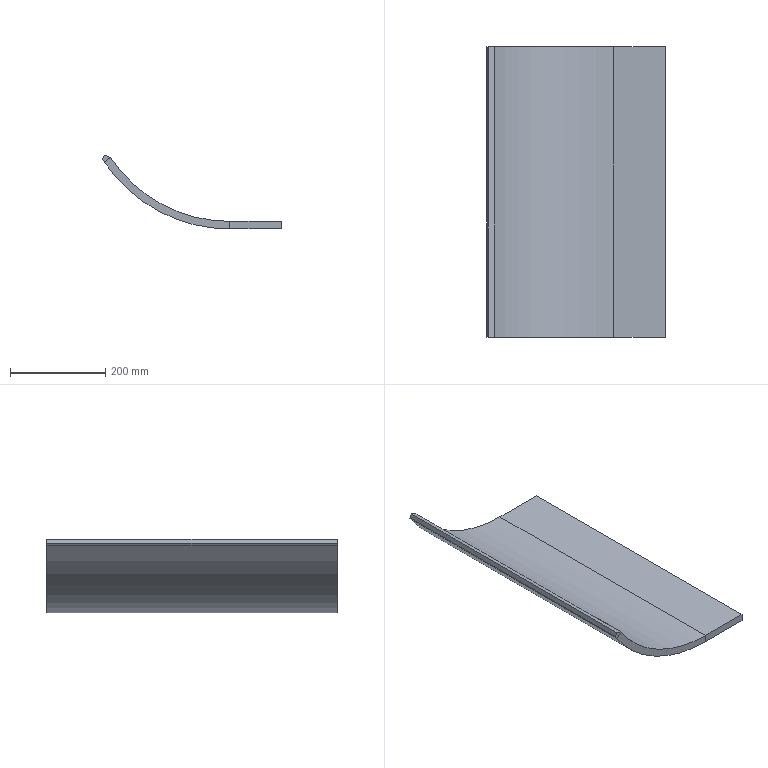Part | SolidWorks | features Chamfer 2, FlatPattern 1, SM3dBend 1, SMBaseFlange 1, SheetMetal 1 | 1 solid | 15 faces | box 375.791 x 610 x 155.275 mm | volume 4096516 mm3 | plane 13 | cylinder 2 | commonest cylinder face diameters 602 x1 634 x1
STEP:
#1=CARTESIAN_POINT('',(64.897,610.,133.992));
#2=VERTEX_POINT('',#1);
#3=CARTESIAN_POINT('',(64.794,610.,134.146));
#4=VERTEX_POINT('',#3);
#5=CARTESIAN_POINT('',(58.413,610.,143.713));
#6=DIRECTION('',(-0.5548,0.,0.832));
#7=VECTOR('',#6,1000.);
#8=LINE('',#5,#7);
#9=EDGE_CURVE('',#2,#4,#8,.T.);
#10=ORIENTED_EDGE('',*,*,#9,.F.);
#11=CARTESIAN_POINT('',(51.585,610.,125.114));
#12=VERTEX_POINT('',#11);
#13=CARTESIAN_POINT('',(51.585,610.,125.114));
#14=DIRECTION('',(-0.832,0.,-0.5548));
#15=VECTOR('',#14,1000.);
#16=LINE('',#13,#15);
#17=EDGE_CURVE('',#2,#12,#16,.T.);
#18=ORIENTED_EDGE('',*,*,#17,.T.);
#19=CARTESIAN_POINT('',(48.209,610.,130.177));
#20=VERTEX_POINT('',#19);
#21=CARTESIAN_POINT('',(45.102,610.,134.836));
#22=DIRECTION('',(-0.5548,0.,0.832));
#23=VECTOR('',#22,1000.);
#24=LINE('',#21,#23);
#25=EDGE_CURVE('',#12,#20,#24,.T.);
#26=ORIENTED_EDGE('',*,*,#25,.T.);
#27=CARTESIAN_POINT('',(51.758,610.,139.275));
#28=VERTEX_POINT('',#27);
#29=CARTESIAN_POINT('',(49.376,610.,133.169));
#30=DIRECTION('',(0.3634,0.,0.9316));
#31=VECTOR('',#30,1000.);
#32=LINE('',#29,#31);
#33=EDGE_CURVE('',#20,#28,#32,.T.);
#34=ORIENTED_EDGE('',*,*,#33,.T.);
#35=CARTESIAN_POINT('',(47.506,610.,140.947));
#36=DIRECTION('',(0.9306,0.,-0.3661));
#37=VECTOR('',#36,1000.);
#38=LINE('',#35,#37);
#39=EDGE_CURVE('',#28,#4,#38,.T.);
#40=ORIENTED_EDGE('',*,*,#39,.T.);
#41=EDGE_LOOP('',(#10,#18,#26,#34,#40));
#42=FACE_OUTER_BOUND('',#41,.T.);
#43=CARTESIAN_POINT('',(45.102,610.,134.836));
#44=DIRECTION('',(0.,1.,0.));
#45=DIRECTION('',(0.832,0.,0.5548));
#46=AXIS2_PLACEMENT_3D('',#43,#44,#45);
#47=PLANE('',#46);
#48=ADVANCED_FACE('',(#42),#47,.T.);
#49=CARTESIAN_POINT('',(48.209,0.,130.177));
#50=VERTEX_POINT('',#49);
#51=CARTESIAN_POINT('',(51.585,0.,125.114));
#52=VERTEX_POINT('',#51);
#53=CARTESIAN_POINT('',(45.102,0.,134.836));
#54=DIRECTION('',(0.5548,0.,-0.832));
#55=VECTOR('',#54,1000.);
#56=LINE('',#53,#55);
#57=EDGE_CURVE('',#50,#52,#56,.T.);
#58=ORIENTED_EDGE('',*,*,#57,.T.);
#59=CARTESIAN_POINT('',(64.897,0.,133.992));
#60=VERTEX_POINT('',#59);
#61=CARTESIAN_POINT('',(51.585,0.,125.114));
#62=DIRECTION('',(0.832,0.,0.5548));
#63=VECTOR('',#62,1000.);
#64=LINE('',#61,#63);
#65=EDGE_CURVE('',#52,#60,#64,.T.);
#66=ORIENTED_EDGE('',*,*,#65,.T.);
#67=CARTESIAN_POINT('',(64.794,0.,134.146));
#68=VERTEX_POINT('',#67);
#69=CARTESIAN_POINT('',(58.413,0.,143.713));
#70=DIRECTION('',(0.5548,0.,-0.832));
#71=VECTOR('',#70,1000.);
#72=LINE('',#69,#71);
#73=EDGE_CURVE('',#68,#60,#72,.T.);
#74=ORIENTED_EDGE('',*,*,#73,.F.);
#75=CARTESIAN_POINT('',(51.758,0.,139.275));
#76=VERTEX_POINT('',#75);
#77=CARTESIAN_POINT('',(47.506,0.,140.947));
#78=DIRECTION('',(-0.9306,0.,0.3661));
#79=VECTOR('',#78,1000.);
#80=LINE('',#77,#79);
#81=EDGE_CURVE('',#68,#76,#80,.T.);
#82=ORIENTED_EDGE('',*,*,#81,.T.);
#83=CARTESIAN_POINT('',(49.376,0.,133.169));
#84=DIRECTION('',(-0.3634,0.,-0.9316));
#85=VECTOR('',#84,1000.);
#86=LINE('',#83,#85);
#87=EDGE_CURVE('',#76,#50,#86,.T.);
#88=ORIENTED_EDGE('',*,*,#87,.T.);
#89=EDGE_LOOP('',(#58,#66,#74,#82,#88));
#90=FACE_OUTER_BOUND('',#89,.T.);
#91=CARTESIAN_POINT('',(45.102,0.,134.836));
#92=DIRECTION('',(0.,-1.,0.));
#93=DIRECTION('',(-0.832,0.,-0.5548));
#94=AXIS2_PLACEMENT_3D('',#91,#92,#93);
#95=PLANE('',#94);
#96=ADVANCED_FACE('',(#90),#95,.T.);
#97=ORIENTED_EDGE('',*,*,#25,.F.);
#98=CARTESIAN_POINT('',(51.585,610.,125.114));
#99=DIRECTION('',(0.,-1.,0.));
#100=VECTOR('',#99,1000.);
#101=LINE('',#98,#100);
#102=EDGE_CURVE('',#12,#52,#101,.T.);
#103=ORIENTED_EDGE('',*,*,#102,.T.);
#104=ORIENTED_EDGE('',*,*,#57,.F.);
#105=CARTESIAN_POINT('',(48.209,610.,130.177));
#106=DIRECTION('',(0.,1.,0.));
#107=VECTOR('',#106,1000.);
#108=LINE('',#105,#107);
#109=EDGE_CURVE('',#50,#20,#108,.T.);
#110=ORIENTED_EDGE('',*,*,#109,.T.);
#111=EDGE_LOOP('',(#97,#103,#104,#110));
#112=FACE_OUTER_BOUND('',#111,.T.);
#113=CARTESIAN_POINT('',(45.102,610.,134.836));
#114=DIRECTION('',(-0.832,0.,-0.5548));
#115=DIRECTION('',(-0.5548,0.,0.832));
#116=AXIS2_PLACEMENT_3D('',#113,#114,#115);
#117=PLANE('',#116);
#118=ADVANCED_FACE('',(#112),#117,.T.);
#119=CARTESIAN_POINT('',(64.897,610.,133.992));
#120=DIRECTION('',(0.,-1.,0.));
#121=VECTOR('',#120,1000.);
#122=LINE('',#119,#121);
#123=EDGE_CURVE('',#2,#60,#122,.T.);
#124=ORIENTED_EDGE('',*,*,#123,.F.);
#125=ORIENTED_EDGE('',*,*,#9,.T.);
#126=CARTESIAN_POINT('',(64.794,0.,134.146));
#127=DIRECTION('',(0.,-1.,0.));
#128=VECTOR('',#127,1000.);
#129=LINE('',#126,#128);
#130=EDGE_CURVE('',#4,#68,#129,.T.);
#131=ORIENTED_EDGE('',*,*,#130,.T.);
#132=ORIENTED_EDGE('',*,*,#73,.T.);
#133=EDGE_LOOP('',(#124,#125,#131,#132));
#134=FACE_OUTER_BOUND('',#133,.T.);
#135=CARTESIAN_POINT('',(58.413,610.,143.713));
#136=DIRECTION('',(-0.832,0.,-0.5548));
#137=DIRECTION('',(-0.5548,0.,0.832));
#138=AXIS2_PLACEMENT_3D('',#135,#136,#137);
#139=PLANE('',#138);
#140=ADVANCED_FACE('',(#134),#139,.F.);
#141=ORIENTED_EDGE('',*,*,#39,.F.);
#142=CARTESIAN_POINT('',(51.758,610.,139.275));
#143=DIRECTION('',(0.,1.,0.));
#144=VECTOR('',#143,1000.);
#145=LINE('',#142,#144);
#146=EDGE_CURVE('',#76,#28,#145,.T.);
#147=ORIENTED_EDGE('',*,*,#146,.F.);
#148=ORIENTED_EDGE('',*,*,#81,.F.);
#149=ORIENTED_EDGE('',*,*,#130,.F.);
#150=EDGE_LOOP('',(#141,#147,#148,#149));
#151=FACE_OUTER_BOUND('',#150,.T.);
#152=CARTESIAN_POINT('',(64.794,610.,134.146));
#153=DIRECTION('',(0.3661,0.,0.9306));
#154=DIRECTION('',(0.9306,0.,-0.3661));
#155=AXIS2_PLACEMENT_3D('',#152,#153,#154);
#156=PLANE('',#155);
#157=ADVANCED_FACE('',(#151),#156,.T.);
#158=ORIENTED_EDGE('',*,*,#33,.F.);
#159=ORIENTED_EDGE('',*,*,#109,.F.);
#160=ORIENTED_EDGE('',*,*,#87,.F.);
#161=ORIENTED_EDGE('',*,*,#146,.T.);
#162=EDGE_LOOP('',(#158,#159,#160,#161));
#163=FACE_OUTER_BOUND('',#162,.T.);
#164=CARTESIAN_POINT('',(51.758,0.,139.275));
#165=DIRECTION('',(0.9316,0.,-0.3634));
#166=DIRECTION('',(-0.3634,0.,-0.9316));
#167=AXIS2_PLACEMENT_3D('',#164,#165,#166);
#168=PLANE('',#167);
#169=ADVANCED_FACE('',(#163),#168,.F.);
#170=CARTESIAN_POINT('',(424.,0.,0.));
#171=VERTEX_POINT('',#170);
#172=CARTESIAN_POINT('',(424.,610.,0.));
#173=VERTEX_POINT('',#172);
#174=CARTESIAN_POINT('',(424.,0.,0.));
#175=DIRECTION('',(0.,1.,0.));
#176=VECTOR('',#175,1000.);
#177=LINE('',#174,#176);
#178=EDGE_CURVE('',#171,#173,#177,.T.);
#179=ORIENTED_EDGE('',*,*,#178,.F.);
#180=CARTESIAN_POINT('',(424.,0.,-16.));
#181=VERTEX_POINT('',#180);
#182=CARTESIAN_POINT('',(424.,0.,-16.));
#183=DIRECTION('',(0.,0.,1.));
#184=VECTOR('',#183,1000.);
#185=LINE('',#182,#184);
#186=EDGE_CURVE('',#181,#171,#185,.T.);
#187=ORIENTED_EDGE('',*,*,#186,.F.);
#188=CARTESIAN_POINT('',(424.,610.,-16.));
#189=VERTEX_POINT('',#188);
#190=CARTESIAN_POINT('',(424.,0.,-16.));
#191=DIRECTION('',(0.,1.,0.));
#192=VECTOR('',#191,1000.);
#193=LINE('',#190,#192);
#194=EDGE_CURVE('',#181,#189,#193,.T.);
#195=ORIENTED_EDGE('',*,*,#194,.T.);
#196=CARTESIAN_POINT('',(424.,610.,-16.));
#197=DIRECTION('',(0.,0.,1.));
#198=VECTOR('',#197,1000.);
#199=LINE('',#196,#198);
#200=EDGE_CURVE('',#189,#173,#199,.T.);
#201=ORIENTED_EDGE('',*,*,#200,.T.);
#202=EDGE_LOOP('',(#179,#187,#195,#201));
#203=FACE_OUTER_BOUND('',#202,.T.);
#204=CARTESIAN_POINT('',(424.,0.,-16.));
#205=DIRECTION('',(1.,0.,0.));
#206=DIRECTION('',(0.,0.,-1.));
#207=AXIS2_PLACEMENT_3D('',#204,#205,#206);
#208=PLANE('',#207);
#209=ADVANCED_FACE('',(#203),#208,.T.);
#210=CARTESIAN_POINT('',(315.315,610.,-16.));
#211=VERTEX_POINT('',#210);
#212=CARTESIAN_POINT('',(315.315,0.,-16.));
#213=VERTEX_POINT('',#212);
#214=CARTESIAN_POINT('',(315.315,610.,-16.));
#215=DIRECTION('',(0.,-1.,0.));
#216=VECTOR('',#215,1000.);
#217=LINE('',#214,#216);
#218=EDGE_CURVE('',#211,#213,#217,.T.);
#219=ORIENTED_EDGE('',*,*,#218,.F.);
#220=CARTESIAN_POINT('',(0.,610.,-16.));
#221=DIRECTION('',(-1.,0.,0.));
#222=VECTOR('',#221,1000.);
#223=LINE('',#220,#222);
#224=EDGE_CURVE('',#189,#211,#223,.T.);
#225=ORIENTED_EDGE('',*,*,#224,.F.);
#226=ORIENTED_EDGE('',*,*,#194,.F.);
#227=CARTESIAN_POINT('',(0.,0.,-16.));
#228=DIRECTION('',(1.,0.,0.));
#229=VECTOR('',#228,1000.);
#230=LINE('',#227,#229);
#231=EDGE_CURVE('',#213,#181,#230,.T.);
#232=ORIENTED_EDGE('',*,*,#231,.F.);
#233=EDGE_LOOP('',(#219,#225,#226,#232));
#234=FACE_OUTER_BOUND('',#233,.T.);
#235=CARTESIAN_POINT('',(0.,610.,-16.));
#236=DIRECTION('',(0.,0.,-1.));
#237=DIRECTION('',(-1.,0.,0.));
#238=AXIS2_PLACEMENT_3D('',#235,#236,#237);
#239=PLANE('',#238);
#240=ADVANCED_FACE('',(#234),#239,.T.);
#241=CARTESIAN_POINT('',(315.315,610.,0.));
#242=VERTEX_POINT('',#241);
#243=CARTESIAN_POINT('',(315.315,610.,-16.));
#244=DIRECTION('',(0.,0.,-1.));
#245=VECTOR('',#244,1000.);
#246=LINE('',#243,#245);
#247=EDGE_CURVE('',#242,#211,#246,.T.);
#248=ORIENTED_EDGE('',*,*,#247,.F.);
#249=CARTESIAN_POINT('',(0.,610.,0.));
#250=DIRECTION('',(-1.,0.,0.));
#251=VECTOR('',#250,1000.);
#252=LINE('',#249,#251);
#253=EDGE_CURVE('',#173,#242,#252,.T.);
#254=ORIENTED_EDGE('',*,*,#253,.F.);
#255=ORIENTED_EDGE('',*,*,#200,.F.);
#256=ORIENTED_EDGE('',*,*,#224,.T.);
#257=EDGE_LOOP('',(#248,#254,#255,#256));
#258=FACE_OUTER_BOUND('',#257,.T.);
#259=CARTESIAN_POINT('',(0.,610.,-16.));
#260=DIRECTION('',(0.,1.,0.));
#261=DIRECTION('',(0.,0.,1.));
#262=AXIS2_PLACEMENT_3D('',#259,#260,#261);
#263=PLANE('',#262);
#264=ADVANCED_FACE('',(#258),#263,.T.);
#265=ORIENTED_EDGE('',*,*,#253,.T.);
#266=CARTESIAN_POINT('',(315.315,0.,0.));
#267=VERTEX_POINT('',#266);
#268=CARTESIAN_POINT('',(315.315,610.,0.));
#269=DIRECTION('',(0.,-1.,0.));
#270=VECTOR('',#269,1000.);
#271=LINE('',#268,#270);
#272=EDGE_CURVE('',#242,#267,#271,.T.);
#273=ORIENTED_EDGE('',*,*,#272,.T.);
#274=CARTESIAN_POINT('',(0.,0.,0.));
#275=DIRECTION('',(1.,0.,0.));
#276=VECTOR('',#275,1000.);
#277=LINE('',#274,#276);
#278=EDGE_CURVE('',#267,#171,#277,.T.);
#279=ORIENTED_EDGE('',*,*,#278,.T.);
#280=ORIENTED_EDGE('',*,*,#178,.T.);
#281=EDGE_LOOP('',(#265,#273,#279,#280));
#282=FACE_OUTER_BOUND('',#281,.T.);
#283=CARTESIAN_POINT('',(0.,610.,0.));
#284=DIRECTION('',(0.,0.,-1.));
#285=DIRECTION('',(-1.,0.,0.));
#286=AXIS2_PLACEMENT_3D('',#283,#284,#285);
#287=PLANE('',#286);
#288=ADVANCED_FACE('',(#282),#287,.F.);
#289=CARTESIAN_POINT('',(315.315,0.,-16.));
#290=DIRECTION('',(0.,0.,1.));
#291=VECTOR('',#290,1000.);
#292=LINE('',#289,#291);
#293=EDGE_CURVE('',#213,#267,#292,.T.);
#294=ORIENTED_EDGE('',*,*,#293,.F.);
#295=ORIENTED_EDGE('',*,*,#231,.T.);
#296=ORIENTED_EDGE('',*,*,#186,.T.);
#297=ORIENTED_EDGE('',*,*,#278,.F.);
#298=EDGE_LOOP('',(#294,#295,#296,#297));
#299=FACE_OUTER_BOUND('',#298,.T.);
#300=CARTESIAN_POINT('',(0.,0.,-16.));
#301=DIRECTION('',(0.,-1.,0.));
#302=DIRECTION('',(0.,0.,-1.));
#303=AXIS2_PLACEMENT_3D('',#300,#301,#302);
#304=PLANE('',#303);
#305=ADVANCED_FACE('',(#299),#304,.T.);
#306=ORIENTED_EDGE('',*,*,#17,.F.);
#307=CARTESIAN_POINT('',(315.315,610.,301.));
#308=DIRECTION('',(0.,-1.,0.));
#309=DIRECTION('',(-1.,0.,0.));
#310=AXIS2_PLACEMENT_3D('',#307,#308,#309);
#311=CIRCLE('',#310,301.);
#312=EDGE_CURVE('',#2,#242,#311,.T.);
#313=ORIENTED_EDGE('',*,*,#312,.T.);
#314=ORIENTED_EDGE('',*,*,#247,.T.);
#315=CARTESIAN_POINT('',(315.315,610.,301.));
#316=DIRECTION('',(0.,-1.,0.));
#317=DIRECTION('',(0.,0.,1.));
#318=AXIS2_PLACEMENT_3D('',#315,#316,#317);
#319=CIRCLE('',#318,317.);
#320=EDGE_CURVE('',#12,#211,#319,.T.);
#321=ORIENTED_EDGE('',*,*,#320,.F.);
#322=EDGE_LOOP('',(#306,#313,#314,#321));
#323=FACE_OUTER_BOUND('',#322,.T.);
#324=CARTESIAN_POINT('',(315.315,610.,301.));
#325=DIRECTION('',(0.,1.,0.));
#326=DIRECTION('',(0.,0.,1.));
#327=AXIS2_PLACEMENT_3D('',#324,#325,#326);
#328=PLANE('',#327);
#329=ADVANCED_FACE('',(#323),#328,.T.);
#330=ORIENTED_EDGE('',*,*,#218,.T.);
#331=CARTESIAN_POINT('',(315.315,0.,301.));
#332=DIRECTION('',(0.,1.,0.));
#333=DIRECTION('',(1.,0.,0.));
#334=AXIS2_PLACEMENT_3D('',#331,#332,#333);
#335=CIRCLE('',#334,317.);
#336=EDGE_CURVE('',#213,#52,#335,.T.);
#337=ORIENTED_EDGE('',*,*,#336,.T.);
#338=ORIENTED_EDGE('',*,*,#102,.F.);
#339=ORIENTED_EDGE('',*,*,#320,.T.);
#340=EDGE_LOOP('',(#330,#337,#338,#339));
#341=FACE_OUTER_BOUND('',#340,.T.);
#342=CARTESIAN_POINT('',(315.315,-376.577,301.));
#343=DIRECTION('',(0.,1.,0.));
#344=DIRECTION('',(-1.,0.,0.));
#345=AXIS2_PLACEMENT_3D('',#342,#343,#344);
#346=CYLINDRICAL_SURFACE('',#345,317.);
#347=ADVANCED_FACE('',(#341),#346,.T.);
#348=CARTESIAN_POINT('',(315.315,0.,301.));
#349=DIRECTION('',(0.,1.,0.));
#350=DIRECTION('',(-1.,0.,0.));
#351=AXIS2_PLACEMENT_3D('',#348,#349,#350);
#352=CIRCLE('',#351,301.);
#353=EDGE_CURVE('',#267,#60,#352,.T.);
#354=ORIENTED_EDGE('',*,*,#353,.T.);
#355=ORIENTED_EDGE('',*,*,#65,.F.);
#356=ORIENTED_EDGE('',*,*,#336,.F.);
#357=ORIENTED_EDGE('',*,*,#293,.T.);
#358=EDGE_LOOP('',(#354,#355,#356,#357));
#359=FACE_OUTER_BOUND('',#358,.T.);
#360=CARTESIAN_POINT('',(315.315,0.,301.));
#361=DIRECTION('',(0.,-1.,0.));
#362=DIRECTION('',(1.,0.,0.));
#363=AXIS2_PLACEMENT_3D('',#360,#361,#362);
#364=PLANE('',#363);
#365=ADVANCED_FACE('',(#359),#364,.T.);
#366=ORIENTED_EDGE('',*,*,#272,.F.);
#367=ORIENTED_EDGE('',*,*,#312,.F.);
#368=ORIENTED_EDGE('',*,*,#123,.T.);
#369=ORIENTED_EDGE('',*,*,#353,.F.);
#370=EDGE_LOOP('',(#366,#367,#368,#369));
#371=FACE_OUTER_BOUND('',#370,.T.);
#372=CARTESIAN_POINT('',(315.315,-376.577,301.));
#373=DIRECTION('',(0.,1.,0.));
#374=DIRECTION('',(-1.,0.,0.));
#375=AXIS2_PLACEMENT_3D('',#372,#373,#374);
#376=CYLINDRICAL_SURFACE('',#375,301.);
#377=ADVANCED_FACE('',(#371),#376,.F.);
#378=CLOSED_SHELL('',(#48,#96,#118,#140,#157,#169,#209,#240,#264,#288,#305,#329,#347,#365,#377));
#379=MANIFOLD_SOLID_BREP('',#378);
#380=CARTESIAN_POINT('',(0.,0.,0.));
#381=DIRECTION('',(0.,0.,1.));
#382=DIRECTION('',(1.,0.,0.));
#383=AXIS2_PLACEMENT_3D('',#380,#381,#382);
#384=(LENGTH_UNIT()NAMED_UNIT(*)SI_UNIT(.MILLI.,.METRE.));
#385=UNCERTAINTY_MEASURE_WITH_UNIT(LENGTH_MEASURE(0.00001),#384,'','');
#386=(NAMED_UNIT(*)PLANE_ANGLE_UNIT()SI_UNIT($,.RADIAN.));
#387=(NAMED_UNIT(*)SI_UNIT($,.STERADIAN.)SOLID_ANGLE_UNIT());
#388=(GEOMETRIC_REPRESENTATION_CONTEXT(3)GLOBAL_UNCERTAINTY_ASSIGNED_CONTEXT((#385))GLOBAL_UNIT_ASSIGNED_CONTEXT((#384,#386,#387))REPRESENTATION_CONTEXT('',''));
#389=ADVANCED_BREP_SHAPE_REPRESENTATION('',(#379,#383),#388);